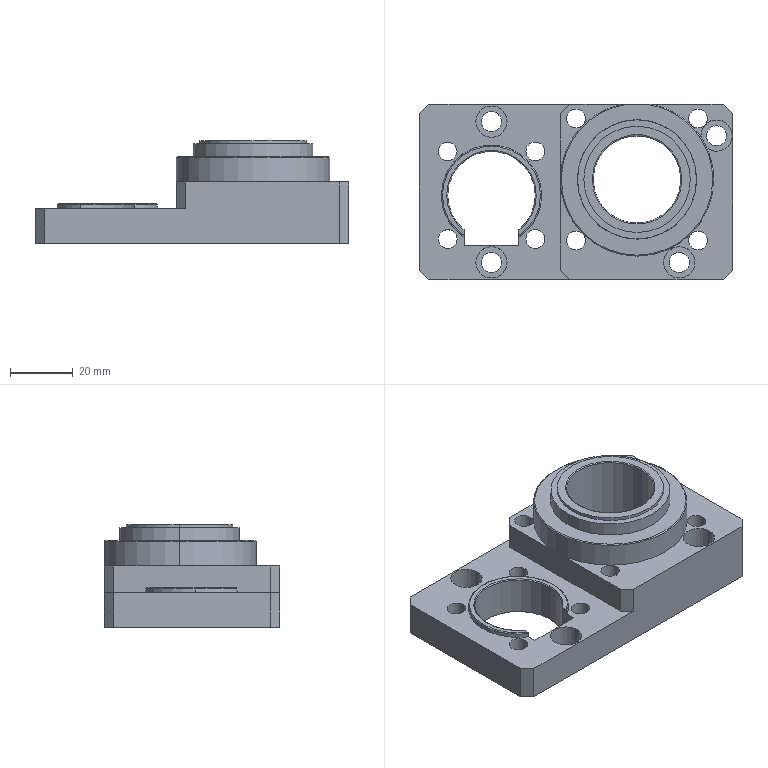Part | SolidWorks | features ICE 6, Cut 3, Fillet 3, Chamfer 1, Extrusion 1, HoleWzd 1 | 1 solid | 85 faces | box 100 x 56 x 32.8 mm | volume 73783 mm3 | cylinder 42 | plane 27 | torus 11 | cone 5 | commonest cylinder face diameters 6 x16 6.4 x8 10 x8 28 x5 49 x3 34 x2